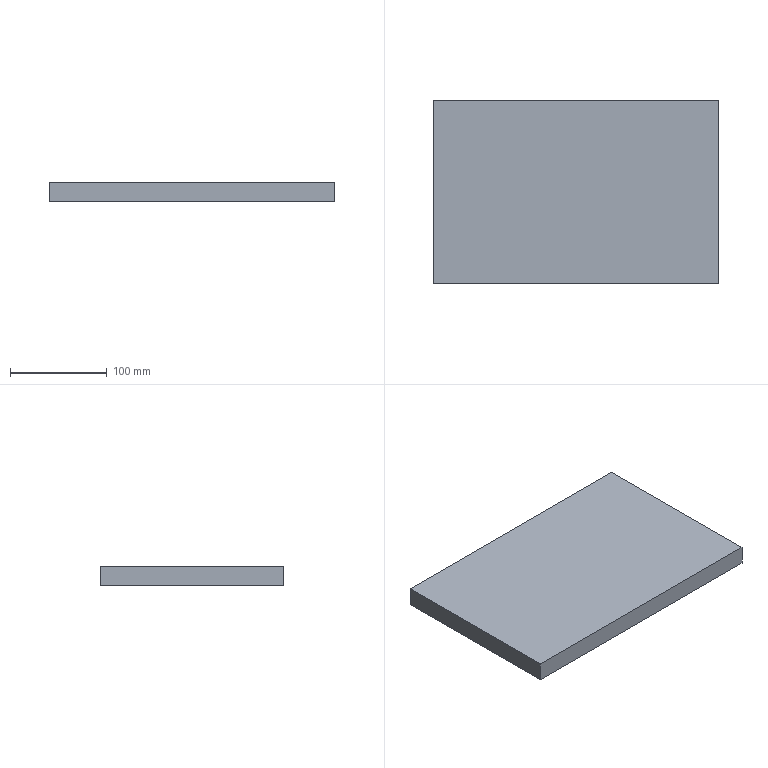Part | STEP file | Tube feed_id770_x_t | 1 solid | 6 faces | box 295 x 190 x 20 mm | volume 1121000 mm3 | plane 6
STEP:
#1=CARTESIAN_POINT('',(0.,0.,0.));
#2=DIRECTION('',(0.,0.,1.));
#3=DIRECTION('',(1.,0.,0.));
#4=AXIS2_PLACEMENT_3D('',#1,#2,#3);
#5=CARTESIAN_POINT('',(326.,305.936,-219.));
#6=VERTEX_POINT('',#5);
#7=CARTESIAN_POINT('',(326.,115.936,-219.));
#8=VERTEX_POINT('',#7);
#9=CARTESIAN_POINT('',(326.,305.936,-219.));
#10=DIRECTION('',(0.,-1.,0.));
#11=VECTOR('',#10,1.);
#12=LINE('',#9,#11);
#13=CARTESIAN_POINT('',(326.,305.936,-199.));
#14=DIRECTION('',(1.,0.,0.));
#15=DIRECTION('',(0.,0.,-1.));
#16=AXIS2_PLACEMENT_3D('',#13,#14,#15);
#17=PLANE('',#16);
#18=CARTESIAN_POINT('',(20.,0.));
#19=DIRECTION('',(0.,-1.));
#20=VECTOR('',#19,1.);
#21=LINE('',#18,#20);
#22=(GEOMETRIC_REPRESENTATION_CONTEXT(2)PARAMETRIC_REPRESENTATION_CONTEXT()REPRESENTATION_CONTEXT('',''));
#23=DEFINITIONAL_REPRESENTATION('',(#21),#22);
#24=PCURVE('',#17,#23);
#25=CARTESIAN_POINT('',(0.,0.,-219.));
#26=DIRECTION('',(0.,0.,1.));
#27=DIRECTION('',(1.,0.,0.));
#28=AXIS2_PLACEMENT_3D('',#25,#26,#27);
#29=PLANE('',#28);
#30=CARTESIAN_POINT('',(326.,305.936));
#31=DIRECTION('',(0.,-1.));
#32=VECTOR('',#31,1.);
#33=LINE('',#30,#32);
#34=(GEOMETRIC_REPRESENTATION_CONTEXT(2)PARAMETRIC_REPRESENTATION_CONTEXT()REPRESENTATION_CONTEXT('',''));
#35=DEFINITIONAL_REPRESENTATION('',(#33),#34);
#36=PCURVE('',#29,#35);
#37=SURFACE_CURVE('',#12,(#24,#36),.PCURVE_S1.);
#38=EDGE_CURVE('',#6,#8,#37,.T.);
#39=ORIENTED_EDGE('',*,*,#38,.T.);
#40=CARTESIAN_POINT('',(326.,115.936,-199.));
#41=VERTEX_POINT('',#40);
#42=CARTESIAN_POINT('',(326.,115.936,-199.));
#43=DIRECTION('',(0.,0.,-1.));
#44=VECTOR('',#43,1.);
#45=LINE('',#42,#44);
#46=CARTESIAN_POINT('',(0.,-190.));
#47=DIRECTION('',(1.,0.));
#48=VECTOR('',#47,1.);
#49=LINE('',#46,#48);
#50=(GEOMETRIC_REPRESENTATION_CONTEXT(2)PARAMETRIC_REPRESENTATION_CONTEXT()REPRESENTATION_CONTEXT('',''));
#51=DEFINITIONAL_REPRESENTATION('',(#49),#50);
#52=PCURVE('',#17,#51);
#53=CARTESIAN_POINT('',(326.,115.936,-199.));
#54=DIRECTION('',(0.,1.,0.));
#55=DIRECTION('',(-1.,0.,0.));
#56=AXIS2_PLACEMENT_3D('',#53,#54,#55);
#57=PLANE('',#56);
#58=CARTESIAN_POINT('',(0.,0.));
#59=DIRECTION('',(0.,-1.));
#60=VECTOR('',#59,1.);
#61=LINE('',#58,#60);
#62=(GEOMETRIC_REPRESENTATION_CONTEXT(2)PARAMETRIC_REPRESENTATION_CONTEXT()REPRESENTATION_CONTEXT('',''));
#63=DEFINITIONAL_REPRESENTATION('',(#61),#62);
#64=PCURVE('',#57,#63);
#65=SURFACE_CURVE('',#45,(#52,#64),.PCURVE_S1.);
#66=EDGE_CURVE('',#41,#8,#65,.T.);
#67=ORIENTED_EDGE('',*,*,#66,.F.);
#68=CARTESIAN_POINT('',(326.,305.936,-199.));
#69=VERTEX_POINT('',#68);
#70=CARTESIAN_POINT('',(326.,305.936,-199.));
#71=DIRECTION('',(0.,-1.,0.));
#72=VECTOR('',#71,1.);
#73=LINE('',#70,#72);
#74=CARTESIAN_POINT('',(0.,0.));
#75=DIRECTION('',(0.,-1.));
#76=VECTOR('',#75,1.);
#77=LINE('',#74,#76);
#78=(GEOMETRIC_REPRESENTATION_CONTEXT(2)PARAMETRIC_REPRESENTATION_CONTEXT()REPRESENTATION_CONTEXT('',''));
#79=DEFINITIONAL_REPRESENTATION('',(#77),#78);
#80=PCURVE('',#17,#79);
#81=CARTESIAN_POINT('',(0.,0.,-199.));
#82=DIRECTION('',(0.,0.,1.));
#83=DIRECTION('',(1.,0.,0.));
#84=AXIS2_PLACEMENT_3D('',#81,#82,#83);
#85=PLANE('',#84);
#86=CARTESIAN_POINT('',(326.,305.936));
#87=DIRECTION('',(0.,-1.));
#88=VECTOR('',#87,1.);
#89=LINE('',#86,#88);
#90=(GEOMETRIC_REPRESENTATION_CONTEXT(2)PARAMETRIC_REPRESENTATION_CONTEXT()REPRESENTATION_CONTEXT('',''));
#91=DEFINITIONAL_REPRESENTATION('',(#89),#90);
#92=PCURVE('',#85,#91);
#93=SURFACE_CURVE('',#73,(#80,#92),.PCURVE_S1.);
#94=EDGE_CURVE('',#69,#41,#93,.T.);
#95=ORIENTED_EDGE('',*,*,#94,.F.);
#96=CARTESIAN_POINT('',(326.,305.936,-199.));
#97=DIRECTION('',(0.,0.,-1.));
#98=VECTOR('',#97,1.);
#99=LINE('',#96,#98);
#100=CARTESIAN_POINT('',(0.,0.));
#101=DIRECTION('',(1.,0.));
#102=VECTOR('',#101,1.);
#103=LINE('',#100,#102);
#104=(GEOMETRIC_REPRESENTATION_CONTEXT(2)PARAMETRIC_REPRESENTATION_CONTEXT()REPRESENTATION_CONTEXT('',''));
#105=DEFINITIONAL_REPRESENTATION('',(#103),#104);
#106=PCURVE('',#17,#105);
#107=CARTESIAN_POINT('',(621.,305.936,-199.));
#108=DIRECTION('',(0.,-1.,0.));
#109=DIRECTION('',(0.,0.,-1.));
#110=AXIS2_PLACEMENT_3D('',#107,#108,#109);
#111=PLANE('',#110);
#112=CARTESIAN_POINT('',(0.,-295.));
#113=DIRECTION('',(1.,0.));
#114=VECTOR('',#113,1.);
#115=LINE('',#112,#114);
#116=(GEOMETRIC_REPRESENTATION_CONTEXT(2)PARAMETRIC_REPRESENTATION_CONTEXT()REPRESENTATION_CONTEXT('',''));
#117=DEFINITIONAL_REPRESENTATION('',(#115),#116);
#118=PCURVE('',#111,#117);
#119=SURFACE_CURVE('',#99,(#106,#118),.PCURVE_S1.);
#120=EDGE_CURVE('',#69,#6,#119,.T.);
#121=ORIENTED_EDGE('',*,*,#120,.T.);
#122=EDGE_LOOP('',(#39,#67,#95,#121));
#123=FACE_BOUND('',#122,.T.);
#124=ADVANCED_FACE('',(#123),#17,.F.);
#125=CARTESIAN_POINT('',(621.,115.936,-219.));
#126=VERTEX_POINT('',#125);
#127=CARTESIAN_POINT('',(326.,115.936,-219.));
#128=DIRECTION('',(1.,0.,0.));
#129=VECTOR('',#128,1.);
#130=LINE('',#127,#129);
#131=CARTESIAN_POINT('',(0.,-20.));
#132=DIRECTION('',(-1.,0.));
#133=VECTOR('',#132,1.);
#134=LINE('',#131,#133);
#135=(GEOMETRIC_REPRESENTATION_CONTEXT(2)PARAMETRIC_REPRESENTATION_CONTEXT()REPRESENTATION_CONTEXT('',''));
#136=DEFINITIONAL_REPRESENTATION('',(#134),#135);
#137=PCURVE('',#57,#136);
#138=CARTESIAN_POINT('',(326.,115.936));
#139=DIRECTION('',(1.,0.));
#140=VECTOR('',#139,1.);
#141=LINE('',#138,#140);
#142=(GEOMETRIC_REPRESENTATION_CONTEXT(2)PARAMETRIC_REPRESENTATION_CONTEXT()REPRESENTATION_CONTEXT('',''));
#143=DEFINITIONAL_REPRESENTATION('',(#141),#142);
#144=PCURVE('',#29,#143);
#145=SURFACE_CURVE('',#130,(#137,#144),.PCURVE_S1.);
#146=EDGE_CURVE('',#8,#126,#145,.T.);
#147=ORIENTED_EDGE('',*,*,#146,.T.);
#148=CARTESIAN_POINT('',(621.,115.936,-199.));
#149=VERTEX_POINT('',#148);
#150=CARTESIAN_POINT('',(621.,115.936,-199.));
#151=DIRECTION('',(0.,0.,-1.));
#152=VECTOR('',#151,1.);
#153=LINE('',#150,#152);
#154=CARTESIAN_POINT('',(-295.,0.));
#155=DIRECTION('',(0.,-1.));
#156=VECTOR('',#155,1.);
#157=LINE('',#154,#156);
#158=(GEOMETRIC_REPRESENTATION_CONTEXT(2)PARAMETRIC_REPRESENTATION_CONTEXT()REPRESENTATION_CONTEXT('',''));
#159=DEFINITIONAL_REPRESENTATION('',(#157),#158);
#160=PCURVE('',#57,#159);
#161=CARTESIAN_POINT('',(621.,115.936,-199.));
#162=DIRECTION('',(-1.,0.,0.));
#163=DIRECTION('',(0.,0.,1.));
#164=AXIS2_PLACEMENT_3D('',#161,#162,#163);
#165=PLANE('',#164);
#166=CARTESIAN_POINT('',(0.,0.));
#167=DIRECTION('',(-1.,0.));
#168=VECTOR('',#167,1.);
#169=LINE('',#166,#168);
#170=(GEOMETRIC_REPRESENTATION_CONTEXT(2)PARAMETRIC_REPRESENTATION_CONTEXT()REPRESENTATION_CONTEXT('',''));
#171=DEFINITIONAL_REPRESENTATION('',(#169),#170);
#172=PCURVE('',#165,#171);
#173=SURFACE_CURVE('',#153,(#160,#172),.PCURVE_S1.);
#174=EDGE_CURVE('',#149,#126,#173,.T.);
#175=ORIENTED_EDGE('',*,*,#174,.F.);
#176=CARTESIAN_POINT('',(326.,115.936,-199.));
#177=DIRECTION('',(1.,0.,0.));
#178=VECTOR('',#177,1.);
#179=LINE('',#176,#178);
#180=CARTESIAN_POINT('',(0.,0.));
#181=DIRECTION('',(-1.,0.));
#182=VECTOR('',#181,1.);
#183=LINE('',#180,#182);
#184=(GEOMETRIC_REPRESENTATION_CONTEXT(2)PARAMETRIC_REPRESENTATION_CONTEXT()REPRESENTATION_CONTEXT('',''));
#185=DEFINITIONAL_REPRESENTATION('',(#183),#184);
#186=PCURVE('',#57,#185);
#187=CARTESIAN_POINT('',(326.,115.936));
#188=DIRECTION('',(1.,0.));
#189=VECTOR('',#188,1.);
#190=LINE('',#187,#189);
#191=(GEOMETRIC_REPRESENTATION_CONTEXT(2)PARAMETRIC_REPRESENTATION_CONTEXT()REPRESENTATION_CONTEXT('',''));
#192=DEFINITIONAL_REPRESENTATION('',(#190),#191);
#193=PCURVE('',#85,#192);
#194=SURFACE_CURVE('',#179,(#186,#193),.PCURVE_S1.);
#195=EDGE_CURVE('',#41,#149,#194,.T.);
#196=ORIENTED_EDGE('',*,*,#195,.F.);
#197=ORIENTED_EDGE('',*,*,#66,.T.);
#198=EDGE_LOOP('',(#147,#175,#196,#197));
#199=FACE_BOUND('',#198,.T.);
#200=ADVANCED_FACE('',(#199),#57,.F.);
#201=CARTESIAN_POINT('',(621.,305.936,-219.));
#202=VERTEX_POINT('',#201);
#203=CARTESIAN_POINT('',(621.,115.936,-219.));
#204=DIRECTION('',(0.,1.,0.));
#205=VECTOR('',#204,1.);
#206=LINE('',#203,#205);
#207=CARTESIAN_POINT('',(-20.,0.));
#208=DIRECTION('',(0.,1.));
#209=VECTOR('',#208,1.);
#210=LINE('',#207,#209);
#211=(GEOMETRIC_REPRESENTATION_CONTEXT(2)PARAMETRIC_REPRESENTATION_CONTEXT()REPRESENTATION_CONTEXT('',''));
#212=DEFINITIONAL_REPRESENTATION('',(#210),#211);
#213=PCURVE('',#165,#212);
#214=CARTESIAN_POINT('',(621.,115.936));
#215=DIRECTION('',(0.,1.));
#216=VECTOR('',#215,1.);
#217=LINE('',#214,#216);
#218=(GEOMETRIC_REPRESENTATION_CONTEXT(2)PARAMETRIC_REPRESENTATION_CONTEXT()REPRESENTATION_CONTEXT('',''));
#219=DEFINITIONAL_REPRESENTATION('',(#217),#218);
#220=PCURVE('',#29,#219);
#221=SURFACE_CURVE('',#206,(#213,#220),.PCURVE_S1.);
#222=EDGE_CURVE('',#126,#202,#221,.T.);
#223=ORIENTED_EDGE('',*,*,#222,.T.);
#224=CARTESIAN_POINT('',(621.,305.936,-199.));
#225=VERTEX_POINT('',#224);
#226=CARTESIAN_POINT('',(621.,305.936,-199.));
#227=DIRECTION('',(0.,0.,-1.));
#228=VECTOR('',#227,1.);
#229=LINE('',#226,#228);
#230=CARTESIAN_POINT('',(0.,190.));
#231=DIRECTION('',(-1.,0.));
#232=VECTOR('',#231,1.);
#233=LINE('',#230,#232);
#234=(GEOMETRIC_REPRESENTATION_CONTEXT(2)PARAMETRIC_REPRESENTATION_CONTEXT()REPRESENTATION_CONTEXT('',''));
#235=DEFINITIONAL_REPRESENTATION('',(#233),#234);
#236=PCURVE('',#165,#235);
#237=CARTESIAN_POINT('',(0.,0.));
#238=DIRECTION('',(1.,0.));
#239=VECTOR('',#238,1.);
#240=LINE('',#237,#239);
#241=(GEOMETRIC_REPRESENTATION_CONTEXT(2)PARAMETRIC_REPRESENTATION_CONTEXT()REPRESENTATION_CONTEXT('',''));
#242=DEFINITIONAL_REPRESENTATION('',(#240),#241);
#243=PCURVE('',#111,#242);
#244=SURFACE_CURVE('',#229,(#236,#243),.PCURVE_S1.);
#245=EDGE_CURVE('',#225,#202,#244,.T.);
#246=ORIENTED_EDGE('',*,*,#245,.F.);
#247=CARTESIAN_POINT('',(621.,115.936,-199.));
#248=DIRECTION('',(0.,1.,0.));
#249=VECTOR('',#248,1.);
#250=LINE('',#247,#249);
#251=CARTESIAN_POINT('',(0.,0.));
#252=DIRECTION('',(0.,1.));
#253=VECTOR('',#252,1.);
#254=LINE('',#251,#253);
#255=(GEOMETRIC_REPRESENTATION_CONTEXT(2)PARAMETRIC_REPRESENTATION_CONTEXT()REPRESENTATION_CONTEXT('',''));
#256=DEFINITIONAL_REPRESENTATION('',(#254),#255);
#257=PCURVE('',#165,#256);
#258=CARTESIAN_POINT('',(621.,115.936));
#259=DIRECTION('',(0.,1.));
#260=VECTOR('',#259,1.);
#261=LINE('',#258,#260);
#262=(GEOMETRIC_REPRESENTATION_CONTEXT(2)PARAMETRIC_REPRESENTATION_CONTEXT()REPRESENTATION_CONTEXT('',''));
#263=DEFINITIONAL_REPRESENTATION('',(#261),#262);
#264=PCURVE('',#85,#263);
#265=SURFACE_CURVE('',#250,(#257,#264),.PCURVE_S1.);
#266=EDGE_CURVE('',#149,#225,#265,.T.);
#267=ORIENTED_EDGE('',*,*,#266,.F.);
#268=ORIENTED_EDGE('',*,*,#174,.T.);
#269=EDGE_LOOP('',(#223,#246,#267,#268));
#270=FACE_BOUND('',#269,.T.);
#271=ADVANCED_FACE('',(#270),#165,.F.);
#272=CARTESIAN_POINT('',(621.,305.936,-219.));
#273=DIRECTION('',(-1.,0.,0.));
#274=VECTOR('',#273,1.);
#275=LINE('',#272,#274);
#276=CARTESIAN_POINT('',(20.,0.));
#277=DIRECTION('',(0.,-1.));
#278=VECTOR('',#277,1.);
#279=LINE('',#276,#278);
#280=(GEOMETRIC_REPRESENTATION_CONTEXT(2)PARAMETRIC_REPRESENTATION_CONTEXT()REPRESENTATION_CONTEXT('',''));
#281=DEFINITIONAL_REPRESENTATION('',(#279),#280);
#282=PCURVE('',#111,#281);
#283=CARTESIAN_POINT('',(621.,305.936));
#284=DIRECTION('',(-1.,0.));
#285=VECTOR('',#284,1.);
#286=LINE('',#283,#285);
#287=(GEOMETRIC_REPRESENTATION_CONTEXT(2)PARAMETRIC_REPRESENTATION_CONTEXT()REPRESENTATION_CONTEXT('',''));
#288=DEFINITIONAL_REPRESENTATION('',(#286),#287);
#289=PCURVE('',#29,#288);
#290=SURFACE_CURVE('',#275,(#282,#289),.PCURVE_S1.);
#291=EDGE_CURVE('',#202,#6,#290,.T.);
#292=ORIENTED_EDGE('',*,*,#291,.T.);
#293=ORIENTED_EDGE('',*,*,#120,.F.);
#294=CARTESIAN_POINT('',(621.,305.936,-199.));
#295=DIRECTION('',(-1.,0.,0.));
#296=VECTOR('',#295,1.);
#297=LINE('',#294,#296);
#298=CARTESIAN_POINT('',(0.,0.));
#299=DIRECTION('',(0.,-1.));
#300=VECTOR('',#299,1.);
#301=LINE('',#298,#300);
#302=(GEOMETRIC_REPRESENTATION_CONTEXT(2)PARAMETRIC_REPRESENTATION_CONTEXT()REPRESENTATION_CONTEXT('',''));
#303=DEFINITIONAL_REPRESENTATION('',(#301),#302);
#304=PCURVE('',#111,#303);
#305=CARTESIAN_POINT('',(621.,305.936));
#306=DIRECTION('',(-1.,0.));
#307=VECTOR('',#306,1.);
#308=LINE('',#305,#307);
#309=(GEOMETRIC_REPRESENTATION_CONTEXT(2)PARAMETRIC_REPRESENTATION_CONTEXT()REPRESENTATION_CONTEXT('',''));
#310=DEFINITIONAL_REPRESENTATION('',(#308),#309);
#311=PCURVE('',#85,#310);
#312=SURFACE_CURVE('',#297,(#304,#311),.PCURVE_S1.);
#313=EDGE_CURVE('',#225,#69,#312,.T.);
#314=ORIENTED_EDGE('',*,*,#313,.F.);
#315=ORIENTED_EDGE('',*,*,#245,.T.);
#316=EDGE_LOOP('',(#292,#293,#314,#315));
#317=FACE_BOUND('',#316,.T.);
#318=ADVANCED_FACE('',(#317),#111,.F.);
#319=ORIENTED_EDGE('',*,*,#94,.T.);
#320=ORIENTED_EDGE('',*,*,#195,.T.);
#321=ORIENTED_EDGE('',*,*,#266,.T.);
#322=ORIENTED_EDGE('',*,*,#313,.T.);
#323=EDGE_LOOP('',(#319,#320,#321,#322));
#324=FACE_BOUND('',#323,.T.);
#325=ADVANCED_FACE('',(#324),#85,.T.);
#326=ORIENTED_EDGE('',*,*,#38,.F.);
#327=ORIENTED_EDGE('',*,*,#291,.F.);
#328=ORIENTED_EDGE('',*,*,#222,.F.);
#329=ORIENTED_EDGE('',*,*,#146,.F.);
#330=EDGE_LOOP('',(#326,#327,#328,#329));
#331=FACE_BOUND('',#330,.T.);
#332=ADVANCED_FACE('',(#331),#29,.F.);
#333=CLOSED_SHELL('',(#124,#200,#271,#318,#325,#332));
#334=MANIFOLD_SOLID_BREP('',#333);
#335=(LENGTH_UNIT()NAMED_UNIT(*)SI_UNIT(.MILLI.,.METRE.));
#336=UNCERTAINTY_MEASURE_WITH_UNIT(LENGTH_MEASURE(0.0000001),#335,'','');
#337=(NAMED_UNIT(*)PLANE_ANGLE_UNIT()SI_UNIT($,.RADIAN.));
#338=(NAMED_UNIT(*)SI_UNIT($,.STERADIAN.)SOLID_ANGLE_UNIT());
#339=(GEOMETRIC_REPRESENTATION_CONTEXT(3)GLOBAL_UNCERTAINTY_ASSIGNED_CONTEXT((#336))GLOBAL_UNIT_ASSIGNED_CONTEXT((#335,#337,#338))REPRESENTATION_CONTEXT('',''));
#340=ADVANCED_BREP_SHAPE_REPRESENTATION('',(#4,#334),#339);